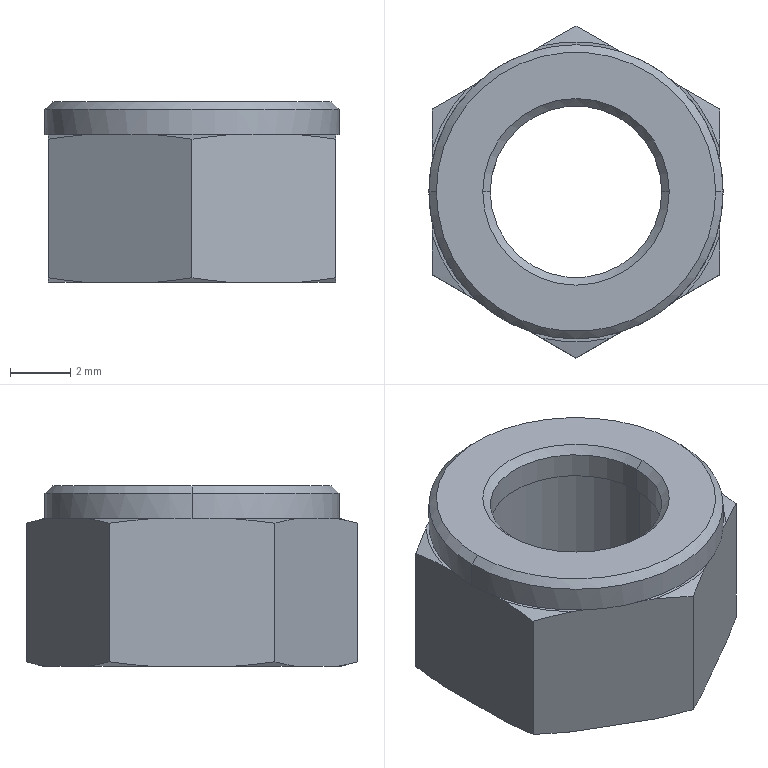Part | SolidWorks | features Cut 3, Boss 1, Chamfer 1, Extrusion 1, MoveFace 1 | 1 solid | 43 faces | box 9.8 x 11.05 x 6 mm | volume 303.009 mm3 | plane 21 | cone 16 | cylinder 6 | commonest cylinder face diameters 5.714 x2 6 x2 9.8 x2
STEP:
#1=CARTESIAN_POINT('',(-2.857,0.,5.75));
#2=VERTEX_POINT('',#1);
#3=CARTESIAN_POINT('',(2.857,0.,5.75));
#4=VERTEX_POINT('',#3);
#5=CARTESIAN_POINT('',(0.,0.,5.75));
#6=DIRECTION('',(0.,0.,1.));
#7=DIRECTION('',(1.,0.,0.));
#8=AXIS2_PLACEMENT_3D('',#5,#6,#7);
#9=CIRCLE('',#8,2.857);
#10=EDGE_CURVE('',#2,#4,#9,.T.);
#11=ORIENTED_EDGE('',*,*,#10,.F.);
#12=CARTESIAN_POINT('',(-3.107,0.,6.));
#13=VERTEX_POINT('',#12);
#14=CARTESIAN_POINT('',(-2.857,0.,5.75));
#15=DIRECTION('',(-0.7071,0.,0.7071));
#16=VECTOR('',#15,1000.);
#17=LINE('',#14,#16);
#18=EDGE_CURVE('',#2,#13,#17,.T.);
#19=ORIENTED_EDGE('',*,*,#18,.T.);
#20=CARTESIAN_POINT('',(3.107,0.,6.));
#21=VERTEX_POINT('',#20);
#22=CARTESIAN_POINT('',(0.,0.,6.));
#23=DIRECTION('',(0.,0.,-1.));
#24=DIRECTION('',(1.,0.,0.));
#25=AXIS2_PLACEMENT_3D('',#22,#23,#24);
#26=CIRCLE('',#25,3.107);
#27=EDGE_CURVE('',#21,#13,#26,.T.);
#28=ORIENTED_EDGE('',*,*,#27,.F.);
#29=CARTESIAN_POINT('',(2.857,0.,5.75));
#30=DIRECTION('',(0.7071,0.,0.7071));
#31=VECTOR('',#30,1000.);
#32=LINE('',#29,#31);
#33=EDGE_CURVE('',#4,#21,#32,.T.);
#34=ORIENTED_EDGE('',*,*,#33,.F.);
#35=EDGE_LOOP('',(#11,#19,#28,#34));
#36=FACE_OUTER_BOUND('',#35,.T.);
#37=CARTESIAN_POINT('',(0.,0.,5.75));
#38=DIRECTION('',(0.,0.,1.));
#39=DIRECTION('',(1.,0.,0.));
#40=AXIS2_PLACEMENT_3D('',#37,#38,#39);
#41=CONICAL_SURFACE('',#40,2.857,0.7854);
#42=ADVANCED_FACE('',(#36),#41,.F.);
#43=CARTESIAN_POINT('',(4.65,0.,6.));
#44=VERTEX_POINT('',#43);
#45=CARTESIAN_POINT('',(-4.65,0.,6.));
#46=VERTEX_POINT('',#45);
#47=CARTESIAN_POINT('',(0.,0.,6.));
#48=DIRECTION('',(0.,0.,1.));
#49=DIRECTION('',(1.,0.,0.));
#50=AXIS2_PLACEMENT_3D('',#47,#48,#49);
#51=CIRCLE('',#50,4.65);
#52=EDGE_CURVE('',#44,#46,#51,.T.);
#53=ORIENTED_EDGE('',*,*,#52,.F.);
#54=CARTESIAN_POINT('',(4.9,0.,5.75));
#55=VERTEX_POINT('',#54);
#56=CARTESIAN_POINT('',(4.65,0.,6.));
#57=DIRECTION('',(0.7071,0.,-0.7071));
#58=VECTOR('',#57,1000.);
#59=LINE('',#56,#58);
#60=EDGE_CURVE('',#44,#55,#59,.T.);
#61=ORIENTED_EDGE('',*,*,#60,.T.);
#62=CARTESIAN_POINT('',(-4.9,0.,5.75));
#63=VERTEX_POINT('',#62);
#64=CARTESIAN_POINT('',(0.,0.,5.75));
#65=DIRECTION('',(0.,0.,-1.));
#66=DIRECTION('',(1.,0.,0.));
#67=AXIS2_PLACEMENT_3D('',#64,#65,#66);
#68=CIRCLE('',#67,4.9);
#69=EDGE_CURVE('',#63,#55,#68,.T.);
#70=ORIENTED_EDGE('',*,*,#69,.F.);
#71=CARTESIAN_POINT('',(-4.65,0.,6.));
#72=DIRECTION('',(-0.7071,0.,-0.7071));
#73=VECTOR('',#72,1000.);
#74=LINE('',#71,#73);
#75=EDGE_CURVE('',#46,#63,#74,.T.);
#76=ORIENTED_EDGE('',*,*,#75,.F.);
#77=EDGE_LOOP('',(#53,#61,#70,#76));
#78=FACE_OUTER_BOUND('',#77,.T.);
#79=CARTESIAN_POINT('',(0.,0.,6.));
#80=DIRECTION('',(0.,0.,-1.));
#81=DIRECTION('',(-1.,0.,0.));
#82=AXIS2_PLACEMENT_3D('',#79,#80,#81);
#83=CONICAL_SURFACE('',#82,4.65,0.7854);
#84=ADVANCED_FACE('',(#78),#83,.T.);
#85=CARTESIAN_POINT('',(-2.857,0.,4.9));
#86=VERTEX_POINT('',#85);
#87=CARTESIAN_POINT('',(2.857,0.,4.9));
#88=VERTEX_POINT('',#87);
#89=CARTESIAN_POINT('',(0.,0.,4.9));
#90=DIRECTION('',(0.,0.,1.));
#91=DIRECTION('',(1.,0.,0.));
#92=AXIS2_PLACEMENT_3D('',#89,#90,#91);
#93=CIRCLE('',#92,2.857);
#94=EDGE_CURVE('',#86,#88,#93,.T.);
#95=ORIENTED_EDGE('',*,*,#94,.F.);
#96=CARTESIAN_POINT('',(-2.857,0.,0.));
#97=DIRECTION('',(0.,0.,1.));
#98=VECTOR('',#97,1000.);
#99=LINE('',#96,#98);
#100=EDGE_CURVE('',#86,#2,#99,.T.);
#101=ORIENTED_EDGE('',*,*,#100,.T.);
#102=ORIENTED_EDGE('',*,*,#10,.T.);
#103=CARTESIAN_POINT('',(2.857,0.,0.));
#104=DIRECTION('',(0.,0.,1.));
#105=VECTOR('',#104,1000.);
#106=LINE('',#103,#105);
#107=EDGE_CURVE('',#88,#4,#106,.T.);
#108=ORIENTED_EDGE('',*,*,#107,.F.);
#109=EDGE_LOOP('',(#95,#101,#102,#108));
#110=FACE_OUTER_BOUND('',#109,.T.);
#111=CARTESIAN_POINT('',(0.,0.,0.));
#112=DIRECTION('',(0.,0.,1.));
#113=DIRECTION('',(1.,0.,0.));
#114=AXIS2_PLACEMENT_3D('',#111,#112,#113);
#115=CYLINDRICAL_SURFACE('',#114,2.857);
#116=ADVANCED_FACE('',(#110),#115,.F.);
#117=ORIENTED_EDGE('',*,*,#69,.T.);
#118=CARTESIAN_POINT('',(4.9,0.,4.9));
#119=VERTEX_POINT('',#118);
#120=CARTESIAN_POINT('',(4.9,0.,8.));
#121=DIRECTION('',(0.,0.,-1.));
#122=VECTOR('',#121,1000.);
#123=LINE('',#120,#122);
#124=EDGE_CURVE('',#55,#119,#123,.T.);
#125=ORIENTED_EDGE('',*,*,#124,.T.);
#126=CARTESIAN_POINT('',(4.785,1.056,4.9));
#127=VERTEX_POINT('',#126);
#128=CARTESIAN_POINT('',(0.,0.,4.9));
#129=DIRECTION('',(0.,0.,1.));
#130=DIRECTION('',(1.,0.,0.));
#131=AXIS2_PLACEMENT_3D('',#128,#129,#130);
#132=CIRCLE('',#131,4.9);
#133=EDGE_CURVE('',#119,#127,#132,.T.);
#134=ORIENTED_EDGE('',*,*,#133,.T.);
#135=CARTESIAN_POINT('',(3.307,3.616,4.9));
#136=VERTEX_POINT('',#135);
#137=CARTESIAN_POINT('',(0.,0.,4.9));
#138=DIRECTION('',(0.,0.,1.));
#139=DIRECTION('',(1.,0.,0.));
#140=AXIS2_PLACEMENT_3D('',#137,#138,#139);
#141=CIRCLE('',#140,4.9);
#142=EDGE_CURVE('',#127,#136,#141,.T.);
#143=ORIENTED_EDGE('',*,*,#142,.T.);
#144=CARTESIAN_POINT('',(1.478,4.672,4.9));
#145=VERTEX_POINT('',#144);
#146=CARTESIAN_POINT('',(0.,0.,4.9));
#147=DIRECTION('',(0.,0.,1.));
#148=DIRECTION('',(1.,0.,0.));
#149=AXIS2_PLACEMENT_3D('',#146,#147,#148);
#150=CIRCLE('',#149,4.9);
#151=EDGE_CURVE('',#136,#145,#150,.T.);
#152=ORIENTED_EDGE('',*,*,#151,.T.);
#153=CARTESIAN_POINT('',(-1.478,4.672,4.9));
#154=VERTEX_POINT('',#153);
#155=CARTESIAN_POINT('',(0.,0.,4.9));
#156=DIRECTION('',(0.,0.,1.));
#157=DIRECTION('',(1.,0.,0.));
#158=AXIS2_PLACEMENT_3D('',#155,#156,#157);
#159=CIRCLE('',#158,4.9);
#160=EDGE_CURVE('',#145,#154,#159,.T.);
#161=ORIENTED_EDGE('',*,*,#160,.T.);
#162=CARTESIAN_POINT('',(-3.307,3.616,4.9));
#163=VERTEX_POINT('',#162);
#164=CARTESIAN_POINT('',(0.,0.,4.9));
#165=DIRECTION('',(0.,0.,1.));
#166=DIRECTION('',(1.,0.,0.));
#167=AXIS2_PLACEMENT_3D('',#164,#165,#166);
#168=CIRCLE('',#167,4.9);
#169=EDGE_CURVE('',#154,#163,#168,.T.);
#170=ORIENTED_EDGE('',*,*,#169,.T.);
#171=CARTESIAN_POINT('',(-4.785,1.056,4.9));
#172=VERTEX_POINT('',#171);
#173=CARTESIAN_POINT('',(0.,0.,4.9));
#174=DIRECTION('',(0.,0.,1.));
#175=DIRECTION('',(1.,0.,0.));
#176=AXIS2_PLACEMENT_3D('',#173,#174,#175);
#177=CIRCLE('',#176,4.9);
#178=EDGE_CURVE('',#163,#172,#177,.T.);
#179=ORIENTED_EDGE('',*,*,#178,.T.);
#180=CARTESIAN_POINT('',(-4.9,0.,4.9));
#181=VERTEX_POINT('',#180);
#182=CARTESIAN_POINT('',(0.,0.,4.9));
#183=DIRECTION('',(0.,0.,1.));
#184=DIRECTION('',(1.,0.,0.));
#185=AXIS2_PLACEMENT_3D('',#182,#183,#184);
#186=CIRCLE('',#185,4.9);
#187=EDGE_CURVE('',#172,#181,#186,.T.);
#188=ORIENTED_EDGE('',*,*,#187,.T.);
#189=CARTESIAN_POINT('',(-4.9,0.,8.));
#190=DIRECTION('',(0.,0.,-1.));
#191=VECTOR('',#190,1000.);
#192=LINE('',#189,#191);
#193=EDGE_CURVE('',#63,#181,#192,.T.);
#194=ORIENTED_EDGE('',*,*,#193,.F.);
#195=EDGE_LOOP('',(#117,#125,#134,#143,#152,#161,#170,#179,#188,#194));
#196=FACE_OUTER_BOUND('',#195,.T.);
#197=CARTESIAN_POINT('',(0.,0.,8.));
#198=DIRECTION('',(0.,0.,-1.));
#199=DIRECTION('',(-1.,0.,0.));
#200=AXIS2_PLACEMENT_3D('',#197,#198,#199);
#201=CYLINDRICAL_SURFACE('',#200,4.9);
#202=ADVANCED_FACE('',(#196),#201,.T.);
#203=CARTESIAN_POINT('',(-3.,0.,4.9));
#204=VERTEX_POINT('',#203);
#205=CARTESIAN_POINT('',(3.,0.,4.9));
#206=VERTEX_POINT('',#205);
#207=CARTESIAN_POINT('',(0.,0.,4.9));
#208=DIRECTION('',(0.,0.,1.));
#209=DIRECTION('',(1.,0.,0.));
#210=AXIS2_PLACEMENT_3D('',#207,#208,#209);
#211=CIRCLE('',#210,3.);
#212=EDGE_CURVE('',#204,#206,#211,.T.);
#213=ORIENTED_EDGE('',*,*,#212,.T.);
#214=CARTESIAN_POINT('',(3.,0.,0.));
#215=VERTEX_POINT('',#214);
#216=CARTESIAN_POINT('',(3.,0.,4.9));
#217=DIRECTION('',(0.,0.,-1.));
#218=VECTOR('',#217,1000.);
#219=LINE('',#216,#218);
#220=EDGE_CURVE('',#206,#215,#219,.T.);
#221=ORIENTED_EDGE('',*,*,#220,.T.);
#222=CARTESIAN_POINT('',(-3.,0.,0.));
#223=VERTEX_POINT('',#222);
#224=CARTESIAN_POINT('',(0.,0.,0.));
#225=DIRECTION('',(0.,0.,1.));
#226=DIRECTION('',(1.,0.,0.));
#227=AXIS2_PLACEMENT_3D('',#224,#225,#226);
#228=CIRCLE('',#227,3.);
#229=EDGE_CURVE('',#223,#215,#228,.T.);
#230=ORIENTED_EDGE('',*,*,#229,.F.);
#231=CARTESIAN_POINT('',(-3.,0.,4.9));
#232=DIRECTION('',(0.,0.,-1.));
#233=VECTOR('',#232,1000.);
#234=LINE('',#231,#233);
#235=EDGE_CURVE('',#204,#223,#234,.T.);
#236=ORIENTED_EDGE('',*,*,#235,.F.);
#237=EDGE_LOOP('',(#213,#221,#230,#236));
#238=FACE_OUTER_BOUND('',#237,.T.);
#239=CARTESIAN_POINT('',(0.,0.,4.9));
#240=DIRECTION('',(0.,0.,-1.));
#241=DIRECTION('',(-1.,0.,0.));
#242=AXIS2_PLACEMENT_3D('',#239,#240,#241);
#243=CYLINDRICAL_SURFACE('',#242,3.);
#244=ADVANCED_FACE('',(#238),#243,.F.);
#245=CARTESIAN_POINT('',(4.785,-1.451,4.9));
#246=VERTEX_POINT('',#245);
#247=CARTESIAN_POINT('',(4.785,-1.056,4.9));
#248=VERTEX_POINT('',#247);
#249=CARTESIAN_POINT('',(4.785,-2.762,4.9));
#250=DIRECTION('',(0.,1.,0.));
#251=VECTOR('',#250,1000.);
#252=LINE('',#249,#251);
#253=EDGE_CURVE('',#246,#248,#252,.T.);
#254=ORIENTED_EDGE('',*,*,#253,.T.);
#255=CARTESIAN_POINT('',(3.307,-3.616,4.9));
#256=VERTEX_POINT('',#255);
#257=CARTESIAN_POINT('',(0.,0.,4.9));
#258=DIRECTION('',(0.,0.,1.));
#259=DIRECTION('',(1.,0.,0.));
#260=AXIS2_PLACEMENT_3D('',#257,#258,#259);
#261=CIRCLE('',#260,4.9);
#262=EDGE_CURVE('',#256,#248,#261,.T.);
#263=ORIENTED_EDGE('',*,*,#262,.F.);
#264=CARTESIAN_POINT('',(3.649,-3.418,4.9));
#265=VERTEX_POINT('',#264);
#266=CARTESIAN_POINT('',(0.,-5.525,4.9));
#267=DIRECTION('',(0.866,0.5,0.));
#268=VECTOR('',#267,1000.);
#269=LINE('',#266,#268);
#270=EDGE_CURVE('',#256,#265,#269,.T.);
#271=ORIENTED_EDGE('',*,*,#270,.T.);
#272=CARTESIAN_POINT('',(0.,0.,4.9));
#273=DIRECTION('',(0.,0.,1.));
#274=DIRECTION('',(1.,0.,0.));
#275=AXIS2_PLACEMENT_3D('',#272,#273,#274);
#276=CIRCLE('',#275,5.);
#277=EDGE_CURVE('',#265,#246,#276,.T.);
#278=ORIENTED_EDGE('',*,*,#277,.T.);
#279=EDGE_LOOP('',(#254,#263,#271,#278));
#280=FACE_OUTER_BOUND('',#279,.T.);
#281=CARTESIAN_POINT('',(-4.785,8.288,4.9));
#282=DIRECTION('',(0.,0.,1.));
#283=DIRECTION('',(1.,0.,0.));
#284=AXIS2_PLACEMENT_3D('',#281,#282,#283);
#285=PLANE('',#284);
#286=ADVANCED_FACE('',(#280),#285,.T.);
#287=CARTESIAN_POINT('',(1.136,-4.869,4.9));
#288=VERTEX_POINT('',#287);
#289=CARTESIAN_POINT('',(1.478,-4.672,4.9));
#290=VERTEX_POINT('',#289);
#291=CARTESIAN_POINT('',(0.,-5.525,4.9));
#292=DIRECTION('',(0.866,0.5,0.));
#293=VECTOR('',#292,1000.);
#294=LINE('',#291,#293);
#295=EDGE_CURVE('',#288,#290,#294,.T.);
#296=ORIENTED_EDGE('',*,*,#295,.T.);
#297=CARTESIAN_POINT('',(-1.478,-4.672,4.9));
#298=VERTEX_POINT('',#297);
#299=CARTESIAN_POINT('',(0.,0.,4.9));
#300=DIRECTION('',(0.,0.,1.));
#301=DIRECTION('',(1.,0.,0.));
#302=AXIS2_PLACEMENT_3D('',#299,#300,#301);
#303=CIRCLE('',#302,4.9);
#304=EDGE_CURVE('',#298,#290,#303,.T.);
#305=ORIENTED_EDGE('',*,*,#304,.F.);
#306=CARTESIAN_POINT('',(-1.136,-4.869,4.9));
#307=VERTEX_POINT('',#306);
#308=CARTESIAN_POINT('',(-4.785,-2.762,4.9));
#309=DIRECTION('',(0.866,-0.5,0.));
#310=VECTOR('',#309,1000.);
#311=LINE('',#308,#310);
#312=EDGE_CURVE('',#298,#307,#311,.T.);
#313=ORIENTED_EDGE('',*,*,#312,.T.);
#314=CARTESIAN_POINT('',(0.,0.,4.9));
#315=DIRECTION('',(0.,0.,1.));
#316=DIRECTION('',(1.,0.,0.));
#317=AXIS2_PLACEMENT_3D('',#314,#315,#316);
#318=CIRCLE('',#317,5.);
#319=EDGE_CURVE('',#307,#288,#318,.T.);
#320=ORIENTED_EDGE('',*,*,#319,.T.);
#321=EDGE_LOOP('',(#296,#305,#313,#320));
#322=FACE_OUTER_BOUND('',#321,.T.);
#323=CARTESIAN_POINT('',(-4.785,8.288,4.9));
#324=DIRECTION('',(0.,0.,1.));
#325=DIRECTION('',(1.,0.,0.));
#326=AXIS2_PLACEMENT_3D('',#323,#324,#325);
#327=PLANE('',#326);
#328=ADVANCED_FACE('',(#322),#327,.T.);
#329=CARTESIAN_POINT('',(-3.649,-3.418,4.9));
#330=VERTEX_POINT('',#329);
#331=CARTESIAN_POINT('',(-3.307,-3.616,4.9));
#332=VERTEX_POINT('',#331);
#333=CARTESIAN_POINT('',(-4.785,-2.762,4.9));
#334=DIRECTION('',(0.866,-0.5,0.));
#335=VECTOR('',#334,1000.);
#336=LINE('',#333,#335);
#337=EDGE_CURVE('',#330,#332,#336,.T.);
#338=ORIENTED_EDGE('',*,*,#337,.T.);
#339=CARTESIAN_POINT('',(-4.785,-1.056,4.9));
#340=VERTEX_POINT('',#339);
#341=CARTESIAN_POINT('',(0.,0.,4.9));
#342=DIRECTION('',(0.,0.,1.));
#343=DIRECTION('',(1.,0.,0.));
#344=AXIS2_PLACEMENT_3D('',#341,#342,#343);
#345=CIRCLE('',#344,4.9);
#346=EDGE_CURVE('',#340,#332,#345,.T.);
#347=ORIENTED_EDGE('',*,*,#346,.F.);
#348=CARTESIAN_POINT('',(-4.785,-1.451,4.9));
#349=VERTEX_POINT('',#348);
#350=CARTESIAN_POINT('',(-4.785,2.763,4.9));
#351=DIRECTION('',(0.,-1.,0.));
#352=VECTOR('',#351,1000.);
#353=LINE('',#350,#352);
#354=EDGE_CURVE('',#340,#349,#353,.T.);
#355=ORIENTED_EDGE('',*,*,#354,.T.);
#356=CARTESIAN_POINT('',(0.,0.,4.9));
#357=DIRECTION('',(0.,0.,1.));
#358=DIRECTION('',(1.,0.,0.));
#359=AXIS2_PLACEMENT_3D('',#356,#357,#358);
#360=CIRCLE('',#359,5.);
#361=EDGE_CURVE('',#349,#330,#360,.T.);
#362=ORIENTED_EDGE('',*,*,#361,.T.);
#363=EDGE_LOOP('',(#338,#347,#355,#362));
#364=FACE_OUTER_BOUND('',#363,.T.);
#365=CARTESIAN_POINT('',(-4.785,8.288,4.9));
#366=DIRECTION('',(0.,0.,1.));
#367=DIRECTION('',(1.,0.,0.));
#368=AXIS2_PLACEMENT_3D('',#365,#366,#367);
#369=PLANE('',#368);
#370=ADVANCED_FACE('',(#364),#369,.T.);
#371=CARTESIAN_POINT('',(-4.785,1.451,4.9));
#372=VERTEX_POINT('',#371);
#373=CARTESIAN_POINT('',(-4.785,2.763,4.9));
#374=DIRECTION('',(0.,-1.,0.));
#375=VECTOR('',#374,1000.);
#376=LINE('',#373,#375);
#377=EDGE_CURVE('',#372,#172,#376,.T.);
#378=ORIENTED_EDGE('',*,*,#377,.T.);
#379=ORIENTED_EDGE('',*,*,#178,.F.);
#380=CARTESIAN_POINT('',(-3.649,3.418,4.9));
#381=VERTEX_POINT('',#380);
#382=CARTESIAN_POINT('',(0.,5.525,4.9));
#383=DIRECTION('',(-0.866,-0.5,0.));
#384=VECTOR('',#383,1000.);
#385=LINE('',#382,#384);
#386=EDGE_CURVE('',#163,#381,#385,.T.);
#387=ORIENTED_EDGE('',*,*,#386,.T.);
#388=CARTESIAN_POINT('',(0.,0.,4.9));
#389=DIRECTION('',(0.,0.,1.));
#390=DIRECTION('',(1.,0.,0.));
#391=AXIS2_PLACEMENT_3D('',#388,#389,#390);
#392=CIRCLE('',#391,5.);
#393=EDGE_CURVE('',#381,#372,#392,.T.);
#394=ORIENTED_EDGE('',*,*,#393,.T.);
#395=EDGE_LOOP('',(#378,#379,#387,#394));
#396=FACE_OUTER_BOUND('',#395,.T.);
#397=CARTESIAN_POINT('',(-4.785,8.288,4.9));
#398=DIRECTION('',(0.,0.,1.));
#399=DIRECTION('',(1.,0.,0.));
#400=AXIS2_PLACEMENT_3D('',#397,#398,#399);
#401=PLANE('',#400);
#402=ADVANCED_FACE('',(#396),#401,.T.);
#403=CARTESIAN_POINT('',(-1.136,4.869,4.9));
#404=VERTEX_POINT('',#403);
#405=CARTESIAN_POINT('',(0.,5.525,4.9));
#406=DIRECTION('',(-0.866,-0.5,0.));
#407=VECTOR('',#406,1000.);
#408=LINE('',#405,#407);
#409=EDGE_CURVE('',#404,#154,#408,.T.);
#410=ORIENTED_EDGE('',*,*,#409,.T.);
#411=ORIENTED_EDGE('',*,*,#160,.F.);
#412=CARTESIAN_POINT('',(1.136,4.869,4.9));
#413=VERTEX_POINT('',#412);
#414=CARTESIAN_POINT('',(4.785,2.763,4.9));
#415=DIRECTION('',(-0.866,0.5,0.));
#416=VECTOR('',#415,1000.);
#417=LINE('',#414,#416);
#418=EDGE_CURVE('',#145,#413,#417,.T.);
#419=ORIENTED_EDGE('',*,*,#418,.T.);
#420=CARTESIAN_POINT('',(0.,0.,4.9));
#421=DIRECTION('',(0.,0.,1.));
#422=DIRECTION('',(1.,0.,0.));
#423=AXIS2_PLACEMENT_3D('',#420,#421,#422);
#424=CIRCLE('',#423,5.);
#425=EDGE_CURVE('',#413,#404,#424,.T.);
#426=ORIENTED_EDGE('',*,*,#425,.T.);
#427=EDGE_LOOP('',(#410,#411,#419,#426));
#428=FACE_OUTER_BOUND('',#427,.T.);
#429=CARTESIAN_POINT('',(-4.785,8.288,4.9));
#430=DIRECTION('',(0.,0.,1.));
#431=DIRECTION('',(1.,0.,0.));
#432=AXIS2_PLACEMENT_3D('',#429,#430,#431);
#433=PLANE('',#432);
#434=ADVANCED_FACE('',(#428),#433,.T.);
#435=CARTESIAN_POINT('',(3.649,3.418,4.9));
#436=VERTEX_POINT('',#435);
#437=CARTESIAN_POINT('',(4.785,2.763,4.9));
#438=DIRECTION('',(-0.866,0.5,0.));
#439=VECTOR('',#438,1000.);
#440=LINE('',#437,#439);
#441=EDGE_CURVE('',#436,#136,#440,.T.);
#442=ORIENTED_EDGE('',*,*,#441,.T.);
#443=ORIENTED_EDGE('',*,*,#142,.F.);
#444=CARTESIAN_POINT('',(4.785,1.451,4.9));
#445=VERTEX_POINT('',#444);
#446=CARTESIAN_POINT('',(4.785,-2.762,4.9));
#447=DIRECTION('',(0.,1.,0.));
#448=VECTOR('',#447,1000.);
#449=LINE('',#446,#448);
#450=EDGE_CURVE('',#127,#445,#449,.T.);
#451=ORIENTED_EDGE('',*,*,#450,.T.);
#452=CARTESIAN_POINT('',(0.,0.,4.9));
#453=DIRECTION('',(0.,0.,1.));
#454=DIRECTION('',(1.,0.,0.));
#455=AXIS2_PLACEMENT_3D('',#452,#453,#454);
#456=CIRCLE('',#455,5.);
#457=EDGE_CURVE('',#445,#436,#456,.T.);
#458=ORIENTED_EDGE('',*,*,#457,.T.);
#459=EDGE_LOOP('',(#442,#443,#451,#458));
#460=FACE_OUTER_BOUND('',#459,.T.);
#461=CARTESIAN_POINT('',(-4.785,8.288,4.9));
#462=DIRECTION('',(0.,0.,1.));
#463=DIRECTION('',(1.,0.,0.));
#464=AXIS2_PLACEMENT_3D('',#461,#462,#463);
#465=PLANE('',#464);
#466=ADVANCED_FACE('',(#460),#465,.T.);
#467=CARTESIAN_POINT('',(0.,5.525,0.1407));
#468=VERTEX_POINT('',#467);
#469=CARTESIAN_POINT('',(1.136,4.869,0.));
#470=VERTEX_POINT('',#469);
#471=CARTESIAN_POINT('',(0.,5.525,0.1407));
#472=CARTESIAN_POINT('',(0.3774,5.307,0.08229));
#473=CARTESIAN_POINT('',(0.7558,5.089,0.03411));
#474=CARTESIAN_POINT('',(1.136,4.869,0.));
#475=B_SPLINE_CURVE_WITH_KNOTS('',3,(#471,#472,#473,#474),.UNSPECIFIED.,.F.,.F.,(4,4),(0.005174,0.006493),.UNSPECIFIED.);
#476=EDGE_CURVE('',#468,#470,#475,.T.);
#477=ORIENTED_EDGE('',*,*,#476,.F.);
#478=CARTESIAN_POINT('',(0.,5.525,4.759));
#479=VERTEX_POINT('',#478);
#480=CARTESIAN_POINT('',(0.,5.525,4.9));
#481=DIRECTION('',(0.,0.,-1.));
#482=VECTOR('',#481,1000.);
#483=LINE('',#480,#482);
#484=EDGE_CURVE('',#479,#468,#483,.T.);
#485=ORIENTED_EDGE('',*,*,#484,.F.);
#486=CARTESIAN_POINT('',(1.136,4.869,4.9));
#487=CARTESIAN_POINT('',(0.7554,5.089,4.866));
#488=CARTESIAN_POINT('',(0.3768,5.307,4.818));
#489=CARTESIAN_POINT('',(0.,5.525,4.759));
#490=B_SPLINE_CURVE_WITH_KNOTS('',3,(#486,#487,#488,#489),.UNSPECIFIED.,.F.,.F.,(4,4),(0.009374,0.01067),.UNSPECIFIED.);
#491=EDGE_CURVE('',#413,#479,#490,.T.);
#492=ORIENTED_EDGE('',*,*,#491,.F.);
#493=ORIENTED_EDGE('',*,*,#418,.F.);
#494=CARTESIAN_POINT('',(4.785,2.763,4.9));
#495=DIRECTION('',(-0.866,0.5,0.));
#496=VECTOR('',#495,1000.);
#497=LINE('',#494,#496);
#498=EDGE_CURVE('',#136,#145,#497,.T.);
#499=ORIENTED_EDGE('',*,*,#498,.F.);
#500=ORIENTED_EDGE('',*,*,#441,.F.);
#501=CARTESIAN_POINT('',(4.785,2.763,4.759));
#502=VERTEX_POINT('',#501);
#503=CARTESIAN_POINT('',(4.785,2.763,4.759));
#504=CARTESIAN_POINT('',(4.407,2.98,4.818));
#505=CARTESIAN_POINT('',(4.029,3.199,4.866));
#506=CARTESIAN_POINT('',(3.649,3.418,4.9));
#507=B_SPLINE_CURVE_WITH_KNOTS('',3,(#503,#504,#505,#506),.UNSPECIFIED.,.F.,.F.,(4,4),(0.005174,0.006493),.UNSPECIFIED.);
#508=EDGE_CURVE('',#502,#436,#507,.T.);
#509=ORIENTED_EDGE('',*,*,#508,.F.);
#510=CARTESIAN_POINT('',(4.785,2.763,0.1407));
#511=VERTEX_POINT('',#510);
#512=CARTESIAN_POINT('',(4.785,2.763,4.9));
#513=DIRECTION('',(0.,0.,-1.));
#514=VECTOR('',#513,1000.);
#515=LINE('',#512,#514);
#516=EDGE_CURVE('',#502,#511,#515,.T.);
#517=ORIENTED_EDGE('',*,*,#516,.T.);
#518=CARTESIAN_POINT('',(3.649,3.418,0.));
#519=VERTEX_POINT('',#518);
#520=CARTESIAN_POINT('',(3.649,3.418,0.));
#521=CARTESIAN_POINT('',(4.029,3.199,0.03415));
#522=CARTESIAN_POINT('',(4.408,2.98,0.08238));
#523=CARTESIAN_POINT('',(4.785,2.763,0.1407));
#524=B_SPLINE_CURVE_WITH_KNOTS('',3,(#520,#521,#522,#523),.UNSPECIFIED.,.F.,.F.,(4,4),(0.009374,0.01067),.UNSPECIFIED.);
#525=EDGE_CURVE('',#519,#511,#524,.T.);
#526=ORIENTED_EDGE('',*,*,#525,.F.);
#527=CARTESIAN_POINT('',(4.785,2.763,0.));
#528=DIRECTION('',(-0.866,0.5,0.));
#529=VECTOR('',#528,1000.);
#530=LINE('',#527,#529);
#531=EDGE_CURVE('',#519,#470,#530,.T.);
#532=ORIENTED_EDGE('',*,*,#531,.T.);
#533=EDGE_LOOP('',(#477,#485,#492,#493,#499,#500,#509,#517,#526,#532));
#534=FACE_OUTER_BOUND('',#533,.T.);
#535=CARTESIAN_POINT('',(4.785,2.763,4.9));
#536=DIRECTION('',(-0.5,-0.866,0.));
#537=DIRECTION('',(0.866,-0.5,0.));
#538=AXIS2_PLACEMENT_3D('',#535,#536,#537);
#539=PLANE('',#538);
#540=ADVANCED_FACE('',(#534),#539,.F.);
#541=CARTESIAN_POINT('',(-4.785,2.763,0.1407));
#542=VERTEX_POINT('',#541);
#543=CARTESIAN_POINT('',(-3.649,3.418,0.));
#544=VERTEX_POINT('',#543);
#545=CARTESIAN_POINT('',(-4.785,2.763,0.1407));
#546=CARTESIAN_POINT('',(-4.407,2.98,0.08229));
#547=CARTESIAN_POINT('',(-4.029,3.199,0.03411));
#548=CARTESIAN_POINT('',(-3.649,3.418,0.));
#549=B_SPLINE_CURVE_WITH_KNOTS('',3,(#545,#546,#547,#548),.UNSPECIFIED.,.F.,.F.,(4,4),(0.005174,0.006493),.UNSPECIFIED.);
#550=EDGE_CURVE('',#542,#544,#549,.T.);
#551=ORIENTED_EDGE('',*,*,#550,.F.);
#552=CARTESIAN_POINT('',(-4.785,2.763,4.759));
#553=VERTEX_POINT('',#552);
#554=CARTESIAN_POINT('',(-4.785,2.763,4.9));
#555=DIRECTION('',(0.,0.,-1.));
#556=VECTOR('',#555,1000.);
#557=LINE('',#554,#556);
#558=EDGE_CURVE('',#553,#542,#557,.T.);
#559=ORIENTED_EDGE('',*,*,#558,.F.);
#560=CARTESIAN_POINT('',(-3.649,3.418,4.9));
#561=CARTESIAN_POINT('',(-4.029,3.199,4.866));
#562=CARTESIAN_POINT('',(-4.408,2.98,4.818));
#563=CARTESIAN_POINT('',(-4.785,2.763,4.759));
#564=B_SPLINE_CURVE_WITH_KNOTS('',3,(#560,#561,#562,#563),.UNSPECIFIED.,.F.,.F.,(4,4),(0.009374,0.01067),.UNSPECIFIED.);
#565=EDGE_CURVE('',#381,#553,#564,.T.);
#566=ORIENTED_EDGE('',*,*,#565,.F.);
#567=ORIENTED_EDGE('',*,*,#386,.F.);
#568=CARTESIAN_POINT('',(0.,5.525,4.9));
#569=DIRECTION('',(-0.866,-0.5,0.));
#570=VECTOR('',#569,1000.);
#571=LINE('',#568,#570);
#572=EDGE_CURVE('',#154,#163,#571,.T.);
#573=ORIENTED_EDGE('',*,*,#572,.F.);
#574=ORIENTED_EDGE('',*,*,#409,.F.);
#575=CARTESIAN_POINT('',(0.,5.525,4.759));
#576=CARTESIAN_POINT('',(-0.3774,5.307,4.818));
#577=CARTESIAN_POINT('',(-0.7558,5.089,4.866));
#578=CARTESIAN_POINT('',(-1.136,4.869,4.9));
#579=B_SPLINE_CURVE_WITH_KNOTS('',3,(#575,#576,#577,#578),.UNSPECIFIED.,.F.,.F.,(4,4),(0.005174,0.006493),.UNSPECIFIED.);
#580=EDGE_CURVE('',#479,#404,#579,.T.);
#581=ORIENTED_EDGE('',*,*,#580,.F.);
#582=ORIENTED_EDGE('',*,*,#484,.T.);
#583=CARTESIAN_POINT('',(-1.136,4.869,0.));
#584=VERTEX_POINT('',#583);
#585=CARTESIAN_POINT('',(-1.136,4.869,0.));
#586=CARTESIAN_POINT('',(-0.7554,5.089,0.03415));
#587=CARTESIAN_POINT('',(-0.3768,5.307,0.08238));
#588=CARTESIAN_POINT('',(0.,5.525,0.1407));
#589=B_SPLINE_CURVE_WITH_KNOTS('',3,(#585,#586,#587,#588),.UNSPECIFIED.,.F.,.F.,(4,4),(0.009374,0.01067),.UNSPECIFIED.);
#590=EDGE_CURVE('',#584,#468,#589,.T.);
#591=ORIENTED_EDGE('',*,*,#590,.F.);
#592=CARTESIAN_POINT('',(0.,5.525,0.));
#593=DIRECTION('',(-0.866,-0.5,0.));
#594=VECTOR('',#593,1000.);
#595=LINE('',#592,#594);
#596=EDGE_CURVE('',#584,#544,#595,.T.);
#597=ORIENTED_EDGE('',*,*,#596,.T.);
#598=EDGE_LOOP('',(#551,#559,#566,#567,#573,#574,#581,#582,#591,#597));
#599=FACE_OUTER_BOUND('',#598,.T.);
#600=CARTESIAN_POINT('',(0.,5.525,4.9));
#601=DIRECTION('',(0.5,-0.866,0.));
#602=DIRECTION('',(0.866,0.5,0.));
#603=AXIS2_PLACEMENT_3D('',#600,#601,#602);
#604=PLANE('',#603);
#605=ADVANCED_FACE('',(#599),#604,.F.);
#606=CARTESIAN_POINT('',(-4.785,-2.762,0.1407));
#607=VERTEX_POINT('',#606);
#608=CARTESIAN_POINT('',(-4.785,-1.451,0.));
#609=VERTEX_POINT('',#608);
#610=CARTESIAN_POINT('',(-4.785,-2.762,0.1407));
#611=CARTESIAN_POINT('',(-4.785,-2.327,0.08228));
#612=CARTESIAN_POINT('',(-4.785,-1.89,0.0341));
#613=CARTESIAN_POINT('',(-4.785,-1.451,0.));
#614=B_SPLINE_CURVE_WITH_KNOTS('',3,(#610,#611,#612,#613),.UNSPECIFIED.,.F.,.F.,(4,4),(0.004475,0.005794),.UNSPECIFIED.);
#615=EDGE_CURVE('',#607,#609,#614,.T.);
#616=ORIENTED_EDGE('',*,*,#615,.F.);
#617=CARTESIAN_POINT('',(-4.785,-2.762,4.759));
#618=VERTEX_POINT('',#617);
#619=CARTESIAN_POINT('',(-4.785,-2.762,4.9));
#620=DIRECTION('',(0.,0.,-1.));
#621=VECTOR('',#620,1000.);
#622=LINE('',#619,#621);
#623=EDGE_CURVE('',#618,#607,#622,.T.);
#624=ORIENTED_EDGE('',*,*,#623,.F.);
#625=CARTESIAN_POINT('',(-4.785,-1.451,4.9));
#626=CARTESIAN_POINT('',(-4.785,-1.89,4.866));
#627=CARTESIAN_POINT('',(-4.785,-2.327,4.818));
#628=CARTESIAN_POINT('',(-4.785,-2.762,4.759));
#629=B_SPLINE_CURVE_WITH_KNOTS('',3,(#625,#626,#627,#628),.UNSPECIFIED.,.F.,.F.,(4,4),(0.008679,0.009975),.UNSPECIFIED.);
#630=EDGE_CURVE('',#349,#618,#629,.T.);
#631=ORIENTED_EDGE('',*,*,#630,.F.);
#632=ORIENTED_EDGE('',*,*,#354,.F.);
#633=CARTESIAN_POINT('',(-4.785,2.763,4.9));
#634=DIRECTION('',(0.,-1.,0.));
#635=VECTOR('',#634,1000.);
#636=LINE('',#633,#635);
#637=EDGE_CURVE('',#172,#340,#636,.T.);
#638=ORIENTED_EDGE('',*,*,#637,.F.);
#639=ORIENTED_EDGE('',*,*,#377,.F.);
#640=CARTESIAN_POINT('',(-4.785,2.763,4.759));
#641=CARTESIAN_POINT('',(-4.785,2.327,4.818));
#642=CARTESIAN_POINT('',(-4.785,1.89,4.866));
#643=CARTESIAN_POINT('',(-4.785,1.451,4.9));
#644=B_SPLINE_CURVE_WITH_KNOTS('',3,(#640,#641,#642,#643),.UNSPECIFIED.,.F.,.F.,(4,4),(0.004475,0.005794),.UNSPECIFIED.);
#645=EDGE_CURVE('',#553,#372,#644,.T.);
#646=ORIENTED_EDGE('',*,*,#645,.F.);
#647=ORIENTED_EDGE('',*,*,#558,.T.);
#648=CARTESIAN_POINT('',(-4.785,1.451,0.));
#649=VERTEX_POINT('',#648);
#650=CARTESIAN_POINT('',(-4.785,1.451,0.));
#651=CARTESIAN_POINT('',(-4.785,1.89,0.0341));
#652=CARTESIAN_POINT('',(-4.785,2.327,0.08237));
#653=CARTESIAN_POINT('',(-4.785,2.763,0.1407));
#654=B_SPLINE_CURVE_WITH_KNOTS('',3,(#650,#651,#652,#653),.UNSPECIFIED.,.F.,.F.,(4,4),(0.008679,0.009975),.UNSPECIFIED.);
#655=EDGE_CURVE('',#649,#542,#654,.T.);
#656=ORIENTED_EDGE('',*,*,#655,.F.);
#657=CARTESIAN_POINT('',(-4.785,2.763,0.));
#658=DIRECTION('',(0.,-1.,0.));
#659=VECTOR('',#658,1000.);
#660=LINE('',#657,#659);
#661=EDGE_CURVE('',#649,#609,#660,.T.);
#662=ORIENTED_EDGE('',*,*,#661,.T.);
#663=EDGE_LOOP('',(#616,#624,#631,#632,#638,#639,#646,#647,#656,#662));
#664=FACE_OUTER_BOUND('',#663,.T.);
#665=CARTESIAN_POINT('',(-4.785,2.763,4.9));
#666=DIRECTION('',(1.,0.,0.));
#667=DIRECTION('',(0.,0.,-1.));
#668=AXIS2_PLACEMENT_3D('',#665,#666,#667);
#669=PLANE('',#668);
#670=ADVANCED_FACE('',(#664),#669,.F.);
#671=CARTESIAN_POINT('',(0.,-5.525,0.1407));
#672=VERTEX_POINT('',#671);
#673=CARTESIAN_POINT('',(-1.136,-4.869,0.));
#674=VERTEX_POINT('',#673);
#675=CARTESIAN_POINT('',(0.,-5.525,0.1407));
#676=CARTESIAN_POINT('',(-0.3774,-5.307,0.08229));
#677=CARTESIAN_POINT('',(-0.7558,-5.089,0.03411));
#678=CARTESIAN_POINT('',(-1.136,-4.869,0.));
#679=B_SPLINE_CURVE_WITH_KNOTS('',3,(#675,#676,#677,#678),.UNSPECIFIED.,.F.,.F.,(4,4),(0.005174,0.006493),.UNSPECIFIED.);
#680=EDGE_CURVE('',#672,#674,#679,.T.);
#681=ORIENTED_EDGE('',*,*,#680,.F.);
#682=CARTESIAN_POINT('',(0.,-5.525,4.759));
#683=VERTEX_POINT('',#682);
#684=CARTESIAN_POINT('',(0.,-5.525,4.9));
#685=DIRECTION('',(0.,0.,-1.));
#686=VECTOR('',#685,1000.);
#687=LINE('',#684,#686);
#688=EDGE_CURVE('',#683,#672,#687,.T.);
#689=ORIENTED_EDGE('',*,*,#688,.F.);
#690=CARTESIAN_POINT('',(-1.136,-4.869,4.9));
#691=CARTESIAN_POINT('',(-0.7554,-5.089,4.866));
#692=CARTESIAN_POINT('',(-0.3768,-5.307,4.818));
#693=CARTESIAN_POINT('',(0.,-5.525,4.759));
#694=B_SPLINE_CURVE_WITH_KNOTS('',3,(#690,#691,#692,#693),.UNSPECIFIED.,.F.,.F.,(4,4),(0.009374,0.01067),.UNSPECIFIED.);
#695=EDGE_CURVE('',#307,#683,#694,.T.);
#696=ORIENTED_EDGE('',*,*,#695,.F.);
#697=ORIENTED_EDGE('',*,*,#312,.F.);
#698=CARTESIAN_POINT('',(-4.785,-2.762,4.9));
#699=DIRECTION('',(0.866,-0.5,0.));
#700=VECTOR('',#699,1000.);
#701=LINE('',#698,#700);
#702=EDGE_CURVE('',#332,#298,#701,.T.);
#703=ORIENTED_EDGE('',*,*,#702,.F.);
#704=ORIENTED_EDGE('',*,*,#337,.F.);
#705=CARTESIAN_POINT('',(-4.785,-2.762,4.759));
#706=CARTESIAN_POINT('',(-4.407,-2.98,4.818));
#707=CARTESIAN_POINT('',(-4.029,-3.199,4.866));
#708=CARTESIAN_POINT('',(-3.649,-3.418,4.9));
#709=B_SPLINE_CURVE_WITH_KNOTS('',3,(#705,#706,#707,#708),.UNSPECIFIED.,.F.,.F.,(4,4),(0.005174,0.006493),.UNSPECIFIED.);
#710=EDGE_CURVE('',#618,#330,#709,.T.);
#711=ORIENTED_EDGE('',*,*,#710,.F.);
#712=ORIENTED_EDGE('',*,*,#623,.T.);
#713=CARTESIAN_POINT('',(-3.649,-3.418,0.));
#714=VERTEX_POINT('',#713);
#715=CARTESIAN_POINT('',(-3.649,-3.418,0.));
#716=CARTESIAN_POINT('',(-4.029,-3.199,0.03415));
#717=CARTESIAN_POINT('',(-4.408,-2.98,0.08238));
#718=CARTESIAN_POINT('',(-4.785,-2.762,0.1407));
#719=B_SPLINE_CURVE_WITH_KNOTS('',3,(#715,#716,#717,#718),.UNSPECIFIED.,.F.,.F.,(4,4),(0.009374,0.01067),.UNSPECIFIED.);
#720=EDGE_CURVE('',#714,#607,#719,.T.);
#721=ORIENTED_EDGE('',*,*,#720,.F.);
#722=CARTESIAN_POINT('',(-4.785,-2.762,0.));
#723=DIRECTION('',(0.866,-0.5,0.));
#724=VECTOR('',#723,1000.);
#725=LINE('',#722,#724);
#726=EDGE_CURVE('',#714,#674,#725,.T.);
#727=ORIENTED_EDGE('',*,*,#726,.T.);
#728=EDGE_LOOP('',(#681,#689,#696,#697,#703,#704,#711,#712,#721,#727));
#729=FACE_OUTER_BOUND('',#728,.T.);
#730=CARTESIAN_POINT('',(-4.785,-2.762,4.9));
#731=DIRECTION('',(0.5,0.866,0.));
#732=DIRECTION('',(-0.866,0.5,0.));
#733=AXIS2_PLACEMENT_3D('',#730,#731,#732);
#734=PLANE('',#733);
#735=ADVANCED_FACE('',(#729),#734,.F.);
#736=CARTESIAN_POINT('',(4.785,-2.763,0.1407));
#737=VERTEX_POINT('',#736);
#738=CARTESIAN_POINT('',(3.649,-3.418,0.));
#739=VERTEX_POINT('',#738);
#740=CARTESIAN_POINT('',(4.785,-2.763,0.1407));
#741=CARTESIAN_POINT('',(4.407,-2.98,0.08229));
#742=CARTESIAN_POINT('',(4.029,-3.199,0.03411));
#743=CARTESIAN_POINT('',(3.649,-3.418,0.));
#744=B_SPLINE_CURVE_WITH_KNOTS('',3,(#740,#741,#742,#743),.UNSPECIFIED.,.F.,.F.,(4,4),(0.005174,0.006493),.UNSPECIFIED.);
#745=EDGE_CURVE('',#737,#739,#744,.T.);
#746=ORIENTED_EDGE('',*,*,#745,.F.);
#747=CARTESIAN_POINT('',(4.785,-2.762,4.759));
#748=VERTEX_POINT('',#747);
#749=CARTESIAN_POINT('',(4.785,-2.762,4.9));
#750=DIRECTION('',(0.,0.,-1.));
#751=VECTOR('',#750,1000.);
#752=LINE('',#749,#751);
#753=EDGE_CURVE('',#748,#737,#752,.T.);
#754=ORIENTED_EDGE('',*,*,#753,.F.);
#755=CARTESIAN_POINT('',(3.649,-3.418,4.9));
#756=CARTESIAN_POINT('',(4.029,-3.199,4.866));
#757=CARTESIAN_POINT('',(4.408,-2.98,4.818));
#758=CARTESIAN_POINT('',(4.785,-2.762,4.759));
#759=B_SPLINE_CURVE_WITH_KNOTS('',3,(#755,#756,#757,#758),.UNSPECIFIED.,.F.,.F.,(4,4),(0.009374,0.01067),.UNSPECIFIED.);
#760=EDGE_CURVE('',#265,#748,#759,.T.);
#761=ORIENTED_EDGE('',*,*,#760,.F.);
#762=ORIENTED_EDGE('',*,*,#270,.F.);
#763=CARTESIAN_POINT('',(0.,-5.525,4.9));
#764=DIRECTION('',(0.866,0.5,0.));
#765=VECTOR('',#764,1000.);
#766=LINE('',#763,#765);
#767=EDGE_CURVE('',#290,#256,#766,.T.);
#768=ORIENTED_EDGE('',*,*,#767,.F.);
#769=ORIENTED_EDGE('',*,*,#295,.F.);
#770=CARTESIAN_POINT('',(0.,-5.525,4.759));
#771=CARTESIAN_POINT('',(0.3774,-5.307,4.818));
#772=CARTESIAN_POINT('',(0.7558,-5.089,4.866));
#773=CARTESIAN_POINT('',(1.136,-4.869,4.9));
#774=B_SPLINE_CURVE_WITH_KNOTS('',3,(#770,#771,#772,#773),.UNSPECIFIED.,.F.,.F.,(4,4),(0.005174,0.006493),.UNSPECIFIED.);
#775=EDGE_CURVE('',#683,#288,#774,.T.);
#776=ORIENTED_EDGE('',*,*,#775,.F.);
#777=ORIENTED_EDGE('',*,*,#688,.T.);
#778=CARTESIAN_POINT('',(1.136,-4.869,0.));
#779=VERTEX_POINT('',#778);
#780=CARTESIAN_POINT('',(1.136,-4.869,0.));
#781=CARTESIAN_POINT('',(0.7554,-5.089,0.03415));
#782=CARTESIAN_POINT('',(0.3768,-5.307,0.08238));
#783=CARTESIAN_POINT('',(0.,-5.525,0.1407));
#784=B_SPLINE_CURVE_WITH_KNOTS('',3,(#780,#781,#782,#783),.UNSPECIFIED.,.F.,.F.,(4,4),(0.009374,0.01067),.UNSPECIFIED.);
#785=EDGE_CURVE('',#779,#672,#784,.T.);
#786=ORIENTED_EDGE('',*,*,#785,.F.);
#787=CARTESIAN_POINT('',(0.,-5.525,0.));
#788=DIRECTION('',(0.866,0.5,0.));
#789=VECTOR('',#788,1000.);
#790=LINE('',#787,#789);
#791=EDGE_CURVE('',#779,#739,#790,.T.);
#792=ORIENTED_EDGE('',*,*,#791,.T.);
#793=EDGE_LOOP('',(#746,#754,#761,#762,#768,#769,#776,#777,#786,#792));
#794=FACE_OUTER_BOUND('',#793,.T.);
#795=CARTESIAN_POINT('',(0.,-5.525,4.9));
#796=DIRECTION('',(-0.5,0.866,0.));
#797=DIRECTION('',(-0.866,-0.5,0.));
#798=AXIS2_PLACEMENT_3D('',#795,#796,#797);
#799=PLANE('',#798);
#800=ADVANCED_FACE('',(#794),#799,.F.);
#801=CARTESIAN_POINT('',(4.785,1.451,0.));
#802=VERTEX_POINT('',#801);
#803=CARTESIAN_POINT('',(4.785,2.763,0.1407));
#804=CARTESIAN_POINT('',(4.785,2.327,0.08228));
#805=CARTESIAN_POINT('',(4.785,1.89,0.0341));
#806=CARTESIAN_POINT('',(4.785,1.451,0.));
#807=B_SPLINE_CURVE_WITH_KNOTS('',3,(#803,#804,#805,#806),.UNSPECIFIED.,.F.,.F.,(4,4),(0.004475,0.005794),.UNSPECIFIED.);
#808=EDGE_CURVE('',#511,#802,#807,.T.);
#809=ORIENTED_EDGE('',*,*,#808,.F.);
#810=ORIENTED_EDGE('',*,*,#516,.F.);
#811=CARTESIAN_POINT('',(4.785,1.451,4.9));
#812=CARTESIAN_POINT('',(4.785,1.89,4.866));
#813=CARTESIAN_POINT('',(4.785,2.327,4.818));
#814=CARTESIAN_POINT('',(4.785,2.763,4.759));
#815=B_SPLINE_CURVE_WITH_KNOTS('',3,(#811,#812,#813,#814),.UNSPECIFIED.,.F.,.F.,(4,4),(0.008679,0.009975),.UNSPECIFIED.);
#816=EDGE_CURVE('',#445,#502,#815,.T.);
#817=ORIENTED_EDGE('',*,*,#816,.F.);
#818=ORIENTED_EDGE('',*,*,#450,.F.);
#819=CARTESIAN_POINT('',(4.785,-2.762,4.9));
#820=DIRECTION('',(0.,1.,0.));
#821=VECTOR('',#820,1000.);
#822=LINE('',#819,#821);
#823=EDGE_CURVE('',#248,#127,#822,.T.);
#824=ORIENTED_EDGE('',*,*,#823,.F.);
#825=ORIENTED_EDGE('',*,*,#253,.F.);
#826=CARTESIAN_POINT('',(4.785,-2.762,4.759));
#827=CARTESIAN_POINT('',(4.785,-2.327,4.818));
#828=CARTESIAN_POINT('',(4.785,-1.89,4.866));
#829=CARTESIAN_POINT('',(4.785,-1.451,4.9));
#830=B_SPLINE_CURVE_WITH_KNOTS('',3,(#826,#827,#828,#829),.UNSPECIFIED.,.F.,.F.,(4,4),(0.004475,0.005794),.UNSPECIFIED.);
#831=EDGE_CURVE('',#748,#246,#830,.T.);
#832=ORIENTED_EDGE('',*,*,#831,.F.);
#833=ORIENTED_EDGE('',*,*,#753,.T.);
#834=CARTESIAN_POINT('',(4.785,-1.451,0.));
#835=VERTEX_POINT('',#834);
#836=CARTESIAN_POINT('',(4.785,-1.451,0.));
#837=CARTESIAN_POINT('',(4.785,-1.89,0.0341));
#838=CARTESIAN_POINT('',(4.785,-2.327,0.08237));
#839=CARTESIAN_POINT('',(4.785,-2.763,0.1407));
#840=B_SPLINE_CURVE_WITH_KNOTS('',3,(#836,#837,#838,#839),.UNSPECIFIED.,.F.,.F.,(4,4),(0.008679,0.009975),.UNSPECIFIED.);
#841=EDGE_CURVE('',#835,#737,#840,.T.);
#842=ORIENTED_EDGE('',*,*,#841,.F.);
#843=CARTESIAN_POINT('',(4.785,-2.762,0.));
#844=DIRECTION('',(0.,1.,0.));
#845=VECTOR('',#844,1000.);
#846=LINE('',#843,#845);
#847=EDGE_CURVE('',#835,#802,#846,.T.);
#848=ORIENTED_EDGE('',*,*,#847,.T.);
#849=EDGE_LOOP('',(#809,#810,#817,#818,#824,#825,#832,#833,#842,#848));
#850=FACE_OUTER_BOUND('',#849,.T.);
#851=CARTESIAN_POINT('',(4.785,-2.762,4.9));
#852=DIRECTION('',(-1.,0.,0.));
#853=DIRECTION('',(0.,0.,1.));
#854=AXIS2_PLACEMENT_3D('',#851,#852,#853);
#855=PLANE('',#854);
#856=ADVANCED_FACE('',(#850),#855,.F.);
#857=ORIENTED_EDGE('',*,*,#229,.T.);
#858=CARTESIAN_POINT('',(0.,0.,0.));
#859=DIRECTION('',(0.,0.,1.));
#860=DIRECTION('',(1.,0.,0.));
#861=AXIS2_PLACEMENT_3D('',#858,#859,#860);
#862=CIRCLE('',#861,3.);
#863=EDGE_CURVE('',#215,#223,#862,.T.);
#864=ORIENTED_EDGE('',*,*,#863,.T.);
#865=EDGE_LOOP('',(#857,#864));
#866=FACE_BOUND('',#865,.T.);
#867=CARTESIAN_POINT('',(0.,0.,0.));
#868=DIRECTION('',(0.,0.,1.));
#869=DIRECTION('',(1.,0.,0.));
#870=AXIS2_PLACEMENT_3D('',#867,#868,#869);
#871=CIRCLE('',#870,5.);
#872=EDGE_CURVE('',#802,#519,#871,.T.);
#873=ORIENTED_EDGE('',*,*,#872,.F.);
#874=ORIENTED_EDGE('',*,*,#847,.F.);
#875=CARTESIAN_POINT('',(0.,0.,0.));
#876=DIRECTION('',(0.,0.,1.));
#877=DIRECTION('',(1.,0.,0.));
#878=AXIS2_PLACEMENT_3D('',#875,#876,#877);
#879=CIRCLE('',#878,5.);
#880=EDGE_CURVE('',#739,#835,#879,.T.);
#881=ORIENTED_EDGE('',*,*,#880,.F.);
#882=ORIENTED_EDGE('',*,*,#791,.F.);
#883=CARTESIAN_POINT('',(0.,0.,0.));
#884=DIRECTION('',(0.,0.,1.));
#885=DIRECTION('',(1.,0.,0.));
#886=AXIS2_PLACEMENT_3D('',#883,#884,#885);
#887=CIRCLE('',#886,5.);
#888=EDGE_CURVE('',#674,#779,#887,.T.);
#889=ORIENTED_EDGE('',*,*,#888,.F.);
#890=ORIENTED_EDGE('',*,*,#726,.F.);
#891=CARTESIAN_POINT('',(0.,0.,0.));
#892=DIRECTION('',(0.,0.,1.));
#893=DIRECTION('',(1.,0.,0.));
#894=AXIS2_PLACEMENT_3D('',#891,#892,#893);
#895=CIRCLE('',#894,5.);
#896=EDGE_CURVE('',#609,#714,#895,.T.);
#897=ORIENTED_EDGE('',*,*,#896,.F.);
#898=ORIENTED_EDGE('',*,*,#661,.F.);
#899=CARTESIAN_POINT('',(0.,0.,0.));
#900=DIRECTION('',(0.,0.,-1.));
#901=DIRECTION('',(-1.,0.,0.));
#902=AXIS2_PLACEMENT_3D('',#899,#900,#901);
#903=CIRCLE('',#902,5.);
#904=EDGE_CURVE('',#649,#544,#903,.T.);
#905=ORIENTED_EDGE('',*,*,#904,.T.);
#906=ORIENTED_EDGE('',*,*,#596,.F.);
#907=CARTESIAN_POINT('',(0.,0.,0.));
#908=DIRECTION('',(0.,0.,1.));
#909=DIRECTION('',(1.,0.,0.));
#910=AXIS2_PLACEMENT_3D('',#907,#908,#909);
#911=CIRCLE('',#910,5.);
#912=EDGE_CURVE('',#470,#584,#911,.T.);
#913=ORIENTED_EDGE('',*,*,#912,.F.);
#914=ORIENTED_EDGE('',*,*,#531,.F.);
#915=EDGE_LOOP('',(#873,#874,#881,#882,#889,#890,#897,#898,#905,#906,#913,#914));
#916=FACE_OUTER_BOUND('',#915,.T.);
#917=CARTESIAN_POINT('',(-4.785,8.288,0.));
#918=DIRECTION('',(0.,0.,1.));
#919=DIRECTION('',(1.,0.,0.));
#920=AXIS2_PLACEMENT_3D('',#917,#918,#919);
#921=PLANE('',#920);
#922=ADVANCED_FACE('',(#866,#916),#921,.F.);
#923=ORIENTED_EDGE('',*,*,#220,.F.);
#924=CARTESIAN_POINT('',(0.,0.,4.9));
#925=DIRECTION('',(0.,0.,1.));
#926=DIRECTION('',(1.,0.,0.));
#927=AXIS2_PLACEMENT_3D('',#924,#925,#926);
#928=CIRCLE('',#927,3.);
#929=EDGE_CURVE('',#206,#204,#928,.T.);
#930=ORIENTED_EDGE('',*,*,#929,.T.);
#931=ORIENTED_EDGE('',*,*,#235,.T.);
#932=ORIENTED_EDGE('',*,*,#863,.F.);
#933=EDGE_LOOP('',(#923,#930,#931,#932));
#934=FACE_OUTER_BOUND('',#933,.T.);
#935=CARTESIAN_POINT('',(0.,0.,4.9));
#936=DIRECTION('',(0.,0.,-1.));
#937=DIRECTION('',(-1.,0.,0.));
#938=AXIS2_PLACEMENT_3D('',#935,#936,#937);
#939=CYLINDRICAL_SURFACE('',#938,3.);
#940=ADVANCED_FACE('',(#934),#939,.F.);
#941=ORIENTED_EDGE('',*,*,#508,.T.);
#942=ORIENTED_EDGE('',*,*,#457,.F.);
#943=ORIENTED_EDGE('',*,*,#816,.T.);
#944=EDGE_LOOP('',(#941,#942,#943));
#945=FACE_OUTER_BOUND('',#944,.T.);
#946=CARTESIAN_POINT('',(0.,0.,4.9));
#947=DIRECTION('',(0.,0.,-1.));
#948=DIRECTION('',(1.,0.,0.));
#949=AXIS2_PLACEMENT_3D('',#946,#947,#948);
#950=CONICAL_SURFACE('',#949,5.,1.309);
#951=ADVANCED_FACE('',(#945),#950,.T.);
#952=ORIENTED_EDGE('',*,*,#760,.T.);
#953=ORIENTED_EDGE('',*,*,#831,.T.);
#954=ORIENTED_EDGE('',*,*,#277,.F.);
#955=EDGE_LOOP('',(#952,#953,#954));
#956=FACE_OUTER_BOUND('',#955,.T.);
#957=CARTESIAN_POINT('',(0.,0.,4.9));
#958=DIRECTION('',(0.,0.,-1.));
#959=DIRECTION('',(1.,0.,0.));
#960=AXIS2_PLACEMENT_3D('',#957,#958,#959);
#961=CONICAL_SURFACE('',#960,5.,1.309);
#962=ADVANCED_FACE('',(#956),#961,.T.);
#963=ORIENTED_EDGE('',*,*,#695,.T.);
#964=ORIENTED_EDGE('',*,*,#775,.T.);
#965=ORIENTED_EDGE('',*,*,#319,.F.);
#966=EDGE_LOOP('',(#963,#964,#965));
#967=FACE_OUTER_BOUND('',#966,.T.);
#968=CARTESIAN_POINT('',(0.,0.,4.9));
#969=DIRECTION('',(0.,0.,-1.));
#970=DIRECTION('',(1.,0.,0.));
#971=AXIS2_PLACEMENT_3D('',#968,#969,#970);
#972=CONICAL_SURFACE('',#971,5.,1.309);
#973=ADVANCED_FACE('',(#967),#972,.T.);
#974=ORIENTED_EDGE('',*,*,#630,.T.);
#975=ORIENTED_EDGE('',*,*,#710,.T.);
#976=ORIENTED_EDGE('',*,*,#361,.F.);
#977=EDGE_LOOP('',(#974,#975,#976));
#978=FACE_OUTER_BOUND('',#977,.T.);
#979=CARTESIAN_POINT('',(0.,0.,4.9));
#980=DIRECTION('',(0.,0.,-1.));
#981=DIRECTION('',(1.,0.,0.));
#982=AXIS2_PLACEMENT_3D('',#979,#980,#981);
#983=CONICAL_SURFACE('',#982,5.,1.309);
#984=ADVANCED_FACE('',(#978),#983,.T.);
#985=ORIENTED_EDGE('',*,*,#565,.T.);
#986=ORIENTED_EDGE('',*,*,#645,.T.);
#987=ORIENTED_EDGE('',*,*,#393,.F.);
#988=EDGE_LOOP('',(#985,#986,#987));
#989=FACE_OUTER_BOUND('',#988,.T.);
#990=CARTESIAN_POINT('',(0.,0.,4.9));
#991=DIRECTION('',(0.,0.,-1.));
#992=DIRECTION('',(1.,0.,0.));
#993=AXIS2_PLACEMENT_3D('',#990,#991,#992);
#994=CONICAL_SURFACE('',#993,5.,1.309);
#995=ADVANCED_FACE('',(#989),#994,.T.);
#996=ORIENTED_EDGE('',*,*,#491,.T.);
#997=ORIENTED_EDGE('',*,*,#580,.T.);
#998=ORIENTED_EDGE('',*,*,#425,.F.);
#999=EDGE_LOOP('',(#996,#997,#998));
#1000=FACE_OUTER_BOUND('',#999,.T.);
#1001=CARTESIAN_POINT('',(0.,0.,4.9));
#1002=DIRECTION('',(0.,0.,-1.));
#1003=DIRECTION('',(1.,0.,0.));
#1004=AXIS2_PLACEMENT_3D('',#1001,#1002,#1003);
#1005=CONICAL_SURFACE('',#1004,5.,1.309);
#1006=ADVANCED_FACE('',(#1000),#1005,.T.);
#1007=ORIENTED_EDGE('',*,*,#745,.T.);
#1008=ORIENTED_EDGE('',*,*,#880,.T.);
#1009=ORIENTED_EDGE('',*,*,#841,.T.);
#1010=EDGE_LOOP('',(#1007,#1008,#1009));
#1011=FACE_OUTER_BOUND('',#1010,.T.);
#1012=CARTESIAN_POINT('',(0.,0.,0.));
#1013=DIRECTION('',(0.,0.,1.));
#1014=DIRECTION('',(-1.,0.,0.));
#1015=AXIS2_PLACEMENT_3D('',#1012,#1013,#1014);
#1016=CONICAL_SURFACE('',#1015,5.,1.309);
#1017=ADVANCED_FACE('',(#1011),#1016,.T.);
#1018=ORIENTED_EDGE('',*,*,#680,.T.);
#1019=ORIENTED_EDGE('',*,*,#888,.T.);
#1020=ORIENTED_EDGE('',*,*,#785,.T.);
#1021=EDGE_LOOP('',(#1018,#1019,#1020));
#1022=FACE_OUTER_BOUND('',#1021,.T.);
#1023=CARTESIAN_POINT('',(0.,0.,0.));
#1024=DIRECTION('',(0.,0.,1.));
#1025=DIRECTION('',(-1.,0.,0.));
#1026=AXIS2_PLACEMENT_3D('',#1023,#1024,#1025);
#1027=CONICAL_SURFACE('',#1026,5.,1.309);
#1028=ADVANCED_FACE('',(#1022),#1027,.T.);
#1029=ORIENTED_EDGE('',*,*,#615,.T.);
#1030=ORIENTED_EDGE('',*,*,#896,.T.);
#1031=ORIENTED_EDGE('',*,*,#720,.T.);
#1032=EDGE_LOOP('',(#1029,#1030,#1031));
#1033=FACE_OUTER_BOUND('',#1032,.T.);
#1034=CARTESIAN_POINT('',(0.,0.,0.));
#1035=DIRECTION('',(0.,0.,1.));
#1036=DIRECTION('',(-1.,0.,0.));
#1037=AXIS2_PLACEMENT_3D('',#1034,#1035,#1036);
#1038=CONICAL_SURFACE('',#1037,5.,1.309);
#1039=ADVANCED_FACE('',(#1033),#1038,.T.);
#1040=ORIENTED_EDGE('',*,*,#550,.T.);
#1041=ORIENTED_EDGE('',*,*,#904,.F.);
#1042=ORIENTED_EDGE('',*,*,#655,.T.);
#1043=EDGE_LOOP('',(#1040,#1041,#1042));
#1044=FACE_OUTER_BOUND('',#1043,.T.);
#1045=CARTESIAN_POINT('',(0.,0.,0.));
#1046=DIRECTION('',(0.,0.,1.));
#1047=DIRECTION('',(-1.,0.,0.));
#1048=AXIS2_PLACEMENT_3D('',#1045,#1046,#1047);
#1049=CONICAL_SURFACE('',#1048,5.,1.309);
#1050=ADVANCED_FACE('',(#1044),#1049,.T.);
#1051=ORIENTED_EDGE('',*,*,#476,.T.);
#1052=ORIENTED_EDGE('',*,*,#912,.T.);
#1053=ORIENTED_EDGE('',*,*,#590,.T.);
#1054=EDGE_LOOP('',(#1051,#1052,#1053));
#1055=FACE_OUTER_BOUND('',#1054,.T.);
#1056=CARTESIAN_POINT('',(0.,0.,0.));
#1057=DIRECTION('',(0.,0.,1.));
#1058=DIRECTION('',(-1.,0.,0.));
#1059=AXIS2_PLACEMENT_3D('',#1056,#1057,#1058);
#1060=CONICAL_SURFACE('',#1059,5.,1.309);
#1061=ADVANCED_FACE('',(#1055),#1060,.T.);
#1062=ORIENTED_EDGE('',*,*,#525,.T.);
#1063=ORIENTED_EDGE('',*,*,#808,.T.);
#1064=ORIENTED_EDGE('',*,*,#872,.T.);
#1065=EDGE_LOOP('',(#1062,#1063,#1064));
#1066=FACE_OUTER_BOUND('',#1065,.T.);
#1067=CARTESIAN_POINT('',(0.,0.,0.));
#1068=DIRECTION('',(0.,0.,1.));
#1069=DIRECTION('',(-1.,0.,0.));
#1070=AXIS2_PLACEMENT_3D('',#1067,#1068,#1069);
#1071=CONICAL_SURFACE('',#1070,5.,1.309);
#1072=ADVANCED_FACE('',(#1066),#1071,.T.);
#1073=CARTESIAN_POINT('',(0.,0.,4.9));
#1074=DIRECTION('',(0.,0.,1.));
#1075=DIRECTION('',(1.,0.,0.));
#1076=AXIS2_PLACEMENT_3D('',#1073,#1074,#1075);
#1077=CIRCLE('',#1076,2.857);
#1078=EDGE_CURVE('',#88,#86,#1077,.T.);
#1079=ORIENTED_EDGE('',*,*,#1078,.T.);
#1080=ORIENTED_EDGE('',*,*,#94,.T.);
#1081=EDGE_LOOP('',(#1079,#1080));
#1082=FACE_BOUND('',#1081,.T.);
#1083=ORIENTED_EDGE('',*,*,#212,.F.);
#1084=ORIENTED_EDGE('',*,*,#929,.F.);
#1085=EDGE_LOOP('',(#1083,#1084));
#1086=FACE_OUTER_BOUND('',#1085,.T.);
#1087=CARTESIAN_POINT('',(0.,0.,4.9));
#1088=DIRECTION('',(0.,0.,1.));
#1089=DIRECTION('',(1.,0.,0.));
#1090=AXIS2_PLACEMENT_3D('',#1087,#1088,#1089);
#1091=PLANE('',#1090);
#1092=ADVANCED_FACE('',(#1082,#1086),#1091,.F.);
#1093=ORIENTED_EDGE('',*,*,#151,.F.);
#1094=ORIENTED_EDGE('',*,*,#498,.T.);
#1095=EDGE_LOOP('',(#1093,#1094));
#1096=FACE_OUTER_BOUND('',#1095,.T.);
#1097=CARTESIAN_POINT('',(0.,0.,4.9));
#1098=DIRECTION('',(0.,0.,1.));
#1099=DIRECTION('',(1.,0.,0.));
#1100=AXIS2_PLACEMENT_3D('',#1097,#1098,#1099);
#1101=PLANE('',#1100);
#1102=ADVANCED_FACE('',(#1096),#1101,.F.);
#1103=ORIENTED_EDGE('',*,*,#169,.F.);
#1104=ORIENTED_EDGE('',*,*,#572,.T.);
#1105=EDGE_LOOP('',(#1103,#1104));
#1106=FACE_OUTER_BOUND('',#1105,.T.);
#1107=CARTESIAN_POINT('',(0.,0.,4.9));
#1108=DIRECTION('',(0.,0.,1.));
#1109=DIRECTION('',(1.,0.,0.));
#1110=AXIS2_PLACEMENT_3D('',#1107,#1108,#1109);
#1111=PLANE('',#1110);
#1112=ADVANCED_FACE('',(#1106),#1111,.F.);
#1113=ORIENTED_EDGE('',*,*,#187,.F.);
#1114=ORIENTED_EDGE('',*,*,#637,.T.);
#1115=CARTESIAN_POINT('',(0.,0.,4.9));
#1116=DIRECTION('',(0.,0.,1.));
#1117=DIRECTION('',(1.,0.,0.));
#1118=AXIS2_PLACEMENT_3D('',#1115,#1116,#1117);
#1119=CIRCLE('',#1118,4.9);
#1120=EDGE_CURVE('',#181,#340,#1119,.T.);
#1121=ORIENTED_EDGE('',*,*,#1120,.F.);
#1122=EDGE_LOOP('',(#1113,#1114,#1121));
#1123=FACE_OUTER_BOUND('',#1122,.T.);
#1124=CARTESIAN_POINT('',(0.,0.,4.9));
#1125=DIRECTION('',(0.,0.,1.));
#1126=DIRECTION('',(1.,0.,0.));
#1127=AXIS2_PLACEMENT_3D('',#1124,#1125,#1126);
#1128=PLANE('',#1127);
#1129=ADVANCED_FACE('',(#1123),#1128,.F.);
#1130=CARTESIAN_POINT('',(0.,0.,4.9));
#1131=DIRECTION('',(0.,0.,1.));
#1132=DIRECTION('',(1.,0.,0.));
#1133=AXIS2_PLACEMENT_3D('',#1130,#1131,#1132);
#1134=CIRCLE('',#1133,4.9);
#1135=EDGE_CURVE('',#332,#298,#1134,.T.);
#1136=ORIENTED_EDGE('',*,*,#1135,.F.);
#1137=ORIENTED_EDGE('',*,*,#702,.T.);
#1138=EDGE_LOOP('',(#1136,#1137));
#1139=FACE_OUTER_BOUND('',#1138,.T.);
#1140=CARTESIAN_POINT('',(0.,0.,4.9));
#1141=DIRECTION('',(0.,0.,1.));
#1142=DIRECTION('',(1.,0.,0.));
#1143=AXIS2_PLACEMENT_3D('',#1140,#1141,#1142);
#1144=PLANE('',#1143);
#1145=ADVANCED_FACE('',(#1139),#1144,.F.);
#1146=CARTESIAN_POINT('',(0.,0.,4.9));
#1147=DIRECTION('',(0.,0.,1.));
#1148=DIRECTION('',(1.,0.,0.));
#1149=AXIS2_PLACEMENT_3D('',#1146,#1147,#1148);
#1150=CIRCLE('',#1149,4.9);
#1151=EDGE_CURVE('',#290,#256,#1150,.T.);
#1152=ORIENTED_EDGE('',*,*,#1151,.F.);
#1153=ORIENTED_EDGE('',*,*,#767,.T.);
#1154=EDGE_LOOP('',(#1152,#1153));
#1155=FACE_OUTER_BOUND('',#1154,.T.);
#1156=CARTESIAN_POINT('',(0.,0.,4.9));
#1157=DIRECTION('',(0.,0.,1.));
#1158=DIRECTION('',(1.,0.,0.));
#1159=AXIS2_PLACEMENT_3D('',#1156,#1157,#1158);
#1160=PLANE('',#1159);
#1161=ADVANCED_FACE('',(#1155),#1160,.F.);
#1162=CARTESIAN_POINT('',(0.,0.,4.9));
#1163=DIRECTION('',(0.,0.,1.));
#1164=DIRECTION('',(1.,0.,0.));
#1165=AXIS2_PLACEMENT_3D('',#1162,#1163,#1164);
#1166=CIRCLE('',#1165,4.9);
#1167=EDGE_CURVE('',#248,#119,#1166,.T.);
#1168=ORIENTED_EDGE('',*,*,#1167,.F.);
#1169=ORIENTED_EDGE('',*,*,#823,.T.);
#1170=ORIENTED_EDGE('',*,*,#133,.F.);
#1171=EDGE_LOOP('',(#1168,#1169,#1170));
#1172=FACE_OUTER_BOUND('',#1171,.T.);
#1173=CARTESIAN_POINT('',(0.,0.,4.9));
#1174=DIRECTION('',(0.,0.,1.));
#1175=DIRECTION('',(1.,0.,0.));
#1176=AXIS2_PLACEMENT_3D('',#1173,#1174,#1175);
#1177=PLANE('',#1176);
#1178=ADVANCED_FACE('',(#1172),#1177,.F.);
#1179=ORIENTED_EDGE('',*,*,#124,.F.);
#1180=CARTESIAN_POINT('',(0.,0.,5.75));
#1181=DIRECTION('',(0.,0.,-1.));
#1182=DIRECTION('',(1.,0.,0.));
#1183=AXIS2_PLACEMENT_3D('',#1180,#1181,#1182);
#1184=CIRCLE('',#1183,4.9);
#1185=EDGE_CURVE('',#55,#63,#1184,.T.);
#1186=ORIENTED_EDGE('',*,*,#1185,.T.);
#1187=ORIENTED_EDGE('',*,*,#193,.T.);
#1188=ORIENTED_EDGE('',*,*,#1120,.T.);
#1189=ORIENTED_EDGE('',*,*,#346,.T.);
#1190=ORIENTED_EDGE('',*,*,#1135,.T.);
#1191=ORIENTED_EDGE('',*,*,#304,.T.);
#1192=ORIENTED_EDGE('',*,*,#1151,.T.);
#1193=ORIENTED_EDGE('',*,*,#262,.T.);
#1194=ORIENTED_EDGE('',*,*,#1167,.T.);
#1195=EDGE_LOOP('',(#1179,#1186,#1187,#1188,#1189,#1190,#1191,#1192,#1193,#1194));
#1196=FACE_OUTER_BOUND('',#1195,.T.);
#1197=CARTESIAN_POINT('',(0.,0.,8.));
#1198=DIRECTION('',(0.,0.,-1.));
#1199=DIRECTION('',(-1.,0.,0.));
#1200=AXIS2_PLACEMENT_3D('',#1197,#1198,#1199);
#1201=CYLINDRICAL_SURFACE('',#1200,4.9);
#1202=ADVANCED_FACE('',(#1196),#1201,.T.);
#1203=CARTESIAN_POINT('',(0.,0.,6.));
#1204=DIRECTION('',(0.,0.,1.));
#1205=DIRECTION('',(1.,0.,0.));
#1206=AXIS2_PLACEMENT_3D('',#1203,#1204,#1205);
#1207=CIRCLE('',#1206,4.65);
#1208=EDGE_CURVE('',#46,#44,#1207,.T.);
#1209=ORIENTED_EDGE('',*,*,#1208,.T.);
#1210=ORIENTED_EDGE('',*,*,#52,.T.);
#1211=EDGE_LOOP('',(#1209,#1210));
#1212=FACE_OUTER_BOUND('',#1211,.T.);
#1213=ORIENTED_EDGE('',*,*,#27,.T.);
#1214=CARTESIAN_POINT('',(0.,0.,6.));
#1215=DIRECTION('',(0.,0.,-1.));
#1216=DIRECTION('',(1.,0.,0.));
#1217=AXIS2_PLACEMENT_3D('',#1214,#1215,#1216);
#1218=CIRCLE('',#1217,3.107);
#1219=EDGE_CURVE('',#13,#21,#1218,.T.);
#1220=ORIENTED_EDGE('',*,*,#1219,.T.);
#1221=EDGE_LOOP('',(#1213,#1220));
#1222=FACE_BOUND('',#1221,.T.);
#1223=CARTESIAN_POINT('',(0.,0.,6.));
#1224=DIRECTION('',(0.,0.,1.));
#1225=DIRECTION('',(1.,0.,0.));
#1226=AXIS2_PLACEMENT_3D('',#1223,#1224,#1225);
#1227=PLANE('',#1226);
#1228=ADVANCED_FACE('',(#1212,#1222),#1227,.T.);
#1229=ORIENTED_EDGE('',*,*,#100,.F.);
#1230=ORIENTED_EDGE('',*,*,#1078,.F.);
#1231=ORIENTED_EDGE('',*,*,#107,.T.);
#1232=CARTESIAN_POINT('',(0.,0.,5.75));
#1233=DIRECTION('',(0.,0.,1.));
#1234=DIRECTION('',(1.,0.,0.));
#1235=AXIS2_PLACEMENT_3D('',#1232,#1233,#1234);
#1236=CIRCLE('',#1235,2.857);
#1237=EDGE_CURVE('',#4,#2,#1236,.T.);
#1238=ORIENTED_EDGE('',*,*,#1237,.T.);
#1239=EDGE_LOOP('',(#1229,#1230,#1231,#1238));
#1240=FACE_OUTER_BOUND('',#1239,.T.);
#1241=CARTESIAN_POINT('',(0.,0.,0.));
#1242=DIRECTION('',(0.,0.,1.));
#1243=DIRECTION('',(1.,0.,0.));
#1244=AXIS2_PLACEMENT_3D('',#1241,#1242,#1243);
#1245=CYLINDRICAL_SURFACE('',#1244,2.857);
#1246=ADVANCED_FACE('',(#1240),#1245,.F.);
#1247=ORIENTED_EDGE('',*,*,#60,.F.);
#1248=ORIENTED_EDGE('',*,*,#1208,.F.);
#1249=ORIENTED_EDGE('',*,*,#75,.T.);
#1250=ORIENTED_EDGE('',*,*,#1185,.F.);
#1251=EDGE_LOOP('',(#1247,#1248,#1249,#1250));
#1252=FACE_OUTER_BOUND('',#1251,.T.);
#1253=CARTESIAN_POINT('',(0.,0.,6.));
#1254=DIRECTION('',(0.,0.,-1.));
#1255=DIRECTION('',(-1.,0.,0.));
#1256=AXIS2_PLACEMENT_3D('',#1253,#1254,#1255);
#1257=CONICAL_SURFACE('',#1256,4.65,0.7854);
#1258=ADVANCED_FACE('',(#1252),#1257,.T.);
#1259=ORIENTED_EDGE('',*,*,#18,.F.);
#1260=ORIENTED_EDGE('',*,*,#1237,.F.);
#1261=ORIENTED_EDGE('',*,*,#33,.T.);
#1262=ORIENTED_EDGE('',*,*,#1219,.F.);
#1263=EDGE_LOOP('',(#1259,#1260,#1261,#1262));
#1264=FACE_OUTER_BOUND('',#1263,.T.);
#1265=CARTESIAN_POINT('',(0.,0.,5.75));
#1266=DIRECTION('',(0.,0.,1.));
#1267=DIRECTION('',(1.,0.,0.));
#1268=AXIS2_PLACEMENT_3D('',#1265,#1266,#1267);
#1269=CONICAL_SURFACE('',#1268,2.857,0.7854);
#1270=ADVANCED_FACE('',(#1264),#1269,.F.);
#1271=CLOSED_SHELL('',(#42,#84,#116,#202,#244,#286,#328,#370,#402,#434,#466,#540,#605,#670,#735,#800,#856,#922,#940,#951,#962,#973,#984,#995,#1006,#1017,#1028,#1039,#1050,#1061,#1072,#1092,#1102,#1112,#1129,#1145,#1161,#1178,#1202,#1228,#1246,#1258,#1270));
#1272=MANIFOLD_SOLID_BREP('',#1271);
#1273=CARTESIAN_POINT('',(0.,0.,0.));
#1274=DIRECTION('',(0.,0.,1.));
#1275=DIRECTION('',(1.,0.,0.));
#1276=AXIS2_PLACEMENT_3D('',#1273,#1274,#1275);
#1277=(LENGTH_UNIT()NAMED_UNIT(*)SI_UNIT(.MILLI.,.METRE.));
#1278=UNCERTAINTY_MEASURE_WITH_UNIT(LENGTH_MEASURE(0.00001),#1277,'','');
#1279=(NAMED_UNIT(*)PLANE_ANGLE_UNIT()SI_UNIT($,.RADIAN.));
#1280=(NAMED_UNIT(*)SI_UNIT($,.STERADIAN.)SOLID_ANGLE_UNIT());
#1281=(GEOMETRIC_REPRESENTATION_CONTEXT(3)GLOBAL_UNCERTAINTY_ASSIGNED_CONTEXT((#1278))GLOBAL_UNIT_ASSIGNED_CONTEXT((#1277,#1279,#1280))REPRESENTATION_CONTEXT('',''));
#1282=ADVANCED_BREP_SHAPE_REPRESENTATION('',(#1272,#1276),#1281);